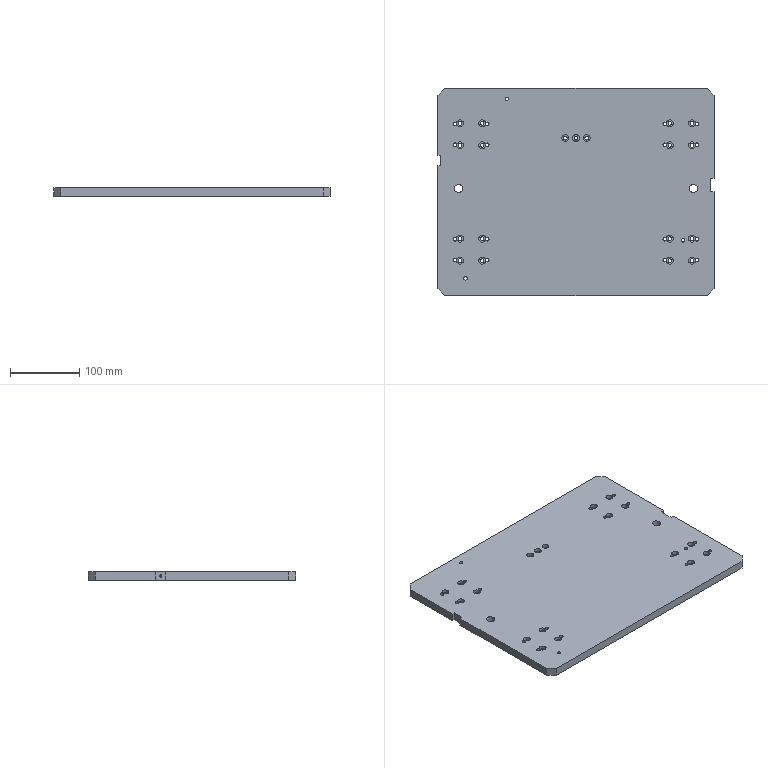Part | NX | features BREP 1 | 1 solid | 175 faces | box 400 x 300 x 12 mm | volume 1416610 mm3 | cylinder 128 | plane 37 | cone 10 | commonest cylinder face diameters 5 x38 5.5 x38 10 x38 2.5 x4 4.2 x4 12 x4